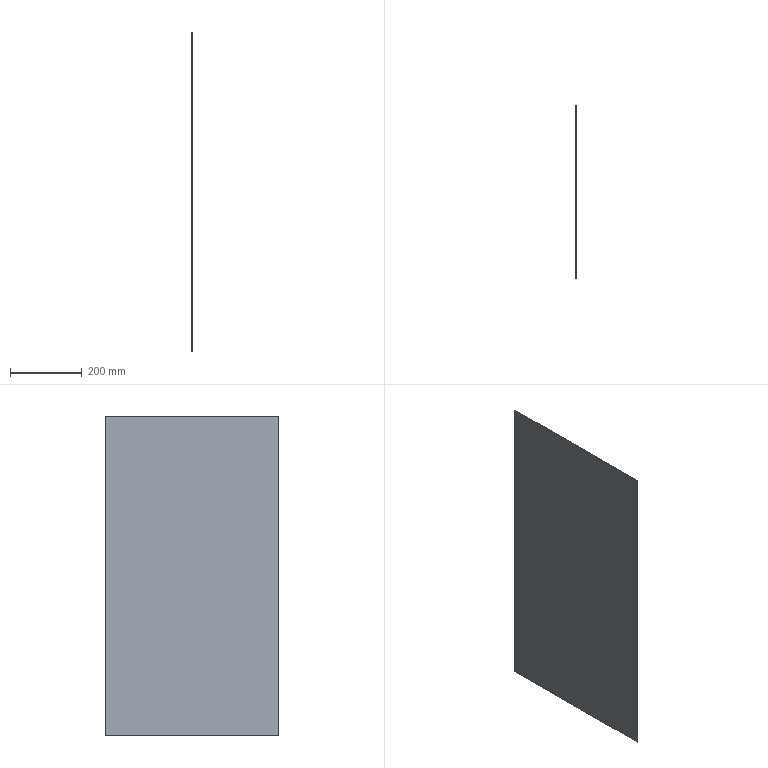Part | STEP file | Guide wheel mechanism revised.sldasm-Part-29 | 1 solid | 6 faces | box 1.2 x 481.99 x 890 mm | volume 514765 mm3 | plane 6
STEP:
#1=CARTESIAN_POINT('',(-485.,1910.,-445.));
#2=VERTEX_POINT('',#1);
#3=CARTESIAN_POINT('',(-485.,1428.01,-445.));
#4=VERTEX_POINT('',#3);
#5=CARTESIAN_POINT('',(-485.,1910.,-445.));
#6=DIRECTION('',(0.,-1.,0.));
#7=VECTOR('',#6,1000.);
#8=LINE('',#5,#7);
#9=EDGE_CURVE('',#2,#4,#8,.T.);
#10=ORIENTED_EDGE('',*,*,#9,.F.);
#11=CARTESIAN_POINT('',(-483.8,1910.,-445.));
#12=VERTEX_POINT('',#11);
#13=CARTESIAN_POINT('',(-483.8,1910.,-445.));
#14=DIRECTION('',(-1.,0.,0.));
#15=VECTOR('',#14,1000.);
#16=LINE('',#13,#15);
#17=EDGE_CURVE('',#12,#2,#16,.T.);
#18=ORIENTED_EDGE('',*,*,#17,.F.);
#19=CARTESIAN_POINT('',(-483.8,1428.01,-445.));
#20=VERTEX_POINT('',#19);
#21=CARTESIAN_POINT('',(-483.8,1910.,-445.));
#22=DIRECTION('',(0.,-1.,0.));
#23=VECTOR('',#22,1000.);
#24=LINE('',#21,#23);
#25=EDGE_CURVE('',#12,#20,#24,.T.);
#26=ORIENTED_EDGE('',*,*,#25,.T.);
#27=CARTESIAN_POINT('',(-483.8,1428.01,-445.));
#28=DIRECTION('',(-1.,0.,0.));
#29=VECTOR('',#28,1000.);
#30=LINE('',#27,#29);
#31=EDGE_CURVE('',#20,#4,#30,.T.);
#32=ORIENTED_EDGE('',*,*,#31,.T.);
#33=EDGE_LOOP('',(#10,#18,#26,#32));
#34=FACE_OUTER_BOUND('',#33,.T.);
#35=CARTESIAN_POINT('',(-483.8,1910.,-445.));
#36=DIRECTION('',(0.,0.,-1.));
#37=DIRECTION('',(0.,1.,0.));
#38=AXIS2_PLACEMENT_3D('',#35,#36,#37);
#39=PLANE('',#38);
#40=ADVANCED_FACE('',(#34),#39,.T.);
#41=CARTESIAN_POINT('',(-485.,1910.,445.));
#42=VERTEX_POINT('',#41);
#43=CARTESIAN_POINT('',(-485.,1910.,-445.));
#44=DIRECTION('',(0.,0.,-1.));
#45=VECTOR('',#44,1000.);
#46=LINE('',#43,#45);
#47=EDGE_CURVE('',#42,#2,#46,.T.);
#48=ORIENTED_EDGE('',*,*,#47,.F.);
#49=CARTESIAN_POINT('',(-483.8,1910.,445.));
#50=VERTEX_POINT('',#49);
#51=CARTESIAN_POINT('',(-483.8,1910.,445.));
#52=DIRECTION('',(-1.,0.,0.));
#53=VECTOR('',#52,1000.);
#54=LINE('',#51,#53);
#55=EDGE_CURVE('',#50,#42,#54,.T.);
#56=ORIENTED_EDGE('',*,*,#55,.F.);
#57=CARTESIAN_POINT('',(-483.8,1910.,-445.));
#58=DIRECTION('',(0.,0.,-1.));
#59=VECTOR('',#58,1000.);
#60=LINE('',#57,#59);
#61=EDGE_CURVE('',#50,#12,#60,.T.);
#62=ORIENTED_EDGE('',*,*,#61,.T.);
#63=ORIENTED_EDGE('',*,*,#17,.T.);
#64=EDGE_LOOP('',(#48,#56,#62,#63));
#65=FACE_OUTER_BOUND('',#64,.T.);
#66=CARTESIAN_POINT('',(-483.8,1910.,-445.));
#67=DIRECTION('',(0.,1.,0.));
#68=DIRECTION('',(0.,0.,1.));
#69=AXIS2_PLACEMENT_3D('',#66,#67,#68);
#70=PLANE('',#69);
#71=ADVANCED_FACE('',(#65),#70,.T.);
#72=CARTESIAN_POINT('',(-485.,1428.01,445.));
#73=VERTEX_POINT('',#72);
#74=CARTESIAN_POINT('',(-485.,1910.,445.));
#75=DIRECTION('',(0.,1.,0.));
#76=VECTOR('',#75,1000.);
#77=LINE('',#74,#76);
#78=EDGE_CURVE('',#73,#42,#77,.T.);
#79=ORIENTED_EDGE('',*,*,#78,.F.);
#80=CARTESIAN_POINT('',(-483.8,1428.01,445.));
#81=VERTEX_POINT('',#80);
#82=CARTESIAN_POINT('',(-483.8,1428.01,445.));
#83=DIRECTION('',(-1.,0.,0.));
#84=VECTOR('',#83,1000.);
#85=LINE('',#82,#84);
#86=EDGE_CURVE('',#81,#73,#85,.T.);
#87=ORIENTED_EDGE('',*,*,#86,.F.);
#88=CARTESIAN_POINT('',(-483.8,1910.,445.));
#89=DIRECTION('',(0.,1.,0.));
#90=VECTOR('',#89,1000.);
#91=LINE('',#88,#90);
#92=EDGE_CURVE('',#81,#50,#91,.T.);
#93=ORIENTED_EDGE('',*,*,#92,.T.);
#94=ORIENTED_EDGE('',*,*,#55,.T.);
#95=EDGE_LOOP('',(#79,#87,#93,#94));
#96=FACE_OUTER_BOUND('',#95,.T.);
#97=CARTESIAN_POINT('',(-483.8,1910.,445.));
#98=DIRECTION('',(0.,0.,1.));
#99=DIRECTION('',(1.,0.,0.));
#100=AXIS2_PLACEMENT_3D('',#97,#98,#99);
#101=PLANE('',#100);
#102=ADVANCED_FACE('',(#96),#101,.T.);
#103=CARTESIAN_POINT('',(-485.,1428.01,-445.));
#104=DIRECTION('',(0.,0.,1.));
#105=VECTOR('',#104,1000.);
#106=LINE('',#103,#105);
#107=EDGE_CURVE('',#4,#73,#106,.T.);
#108=ORIENTED_EDGE('',*,*,#107,.F.);
#109=ORIENTED_EDGE('',*,*,#31,.F.);
#110=CARTESIAN_POINT('',(-483.8,1428.01,-445.));
#111=DIRECTION('',(0.,0.,1.));
#112=VECTOR('',#111,1000.);
#113=LINE('',#110,#112);
#114=EDGE_CURVE('',#20,#81,#113,.T.);
#115=ORIENTED_EDGE('',*,*,#114,.T.);
#116=ORIENTED_EDGE('',*,*,#86,.T.);
#117=EDGE_LOOP('',(#108,#109,#115,#116));
#118=FACE_OUTER_BOUND('',#117,.T.);
#119=CARTESIAN_POINT('',(-483.8,1428.01,-445.));
#120=DIRECTION('',(0.,-1.,0.));
#121=DIRECTION('',(0.,0.,-1.));
#122=AXIS2_PLACEMENT_3D('',#119,#120,#121);
#123=PLANE('',#122);
#124=ADVANCED_FACE('',(#118),#123,.T.);
#125=ORIENTED_EDGE('',*,*,#25,.F.);
#126=ORIENTED_EDGE('',*,*,#61,.F.);
#127=ORIENTED_EDGE('',*,*,#92,.F.);
#128=ORIENTED_EDGE('',*,*,#114,.F.);
#129=EDGE_LOOP('',(#125,#126,#127,#128));
#130=FACE_OUTER_BOUND('',#129,.T.);
#131=CARTESIAN_POINT('',(-483.8,0.,0.));
#132=DIRECTION('',(-1.,0.,0.));
#133=DIRECTION('',(0.,0.,1.));
#134=AXIS2_PLACEMENT_3D('',#131,#132,#133);
#135=PLANE('',#134);
#136=ADVANCED_FACE('',(#130),#135,.F.);
#137=ORIENTED_EDGE('',*,*,#9,.T.);
#138=ORIENTED_EDGE('',*,*,#107,.T.);
#139=ORIENTED_EDGE('',*,*,#78,.T.);
#140=ORIENTED_EDGE('',*,*,#47,.T.);
#141=EDGE_LOOP('',(#137,#138,#139,#140));
#142=FACE_OUTER_BOUND('',#141,.T.);
#143=CARTESIAN_POINT('',(-485.,0.,0.));
#144=DIRECTION('',(-1.,0.,0.));
#145=DIRECTION('',(0.,0.,1.));
#146=AXIS2_PLACEMENT_3D('',#143,#144,#145);
#147=PLANE('',#146);
#148=ADVANCED_FACE('',(#142),#147,.T.);
#149=CLOSED_SHELL('',(#40,#71,#102,#124,#136,#148));
#150=MANIFOLD_SOLID_BREP('',#149);
#151=CARTESIAN_POINT('',(0.,0.,0.));
#152=DIRECTION('',(0.,0.,1.));
#153=DIRECTION('',(1.,0.,0.));
#154=AXIS2_PLACEMENT_3D('',#151,#152,#153);
#155=(LENGTH_UNIT()NAMED_UNIT(*)SI_UNIT(.MILLI.,.METRE.));
#156=UNCERTAINTY_MEASURE_WITH_UNIT(LENGTH_MEASURE(0.00001),#155,'','');
#157=(NAMED_UNIT(*)PLANE_ANGLE_UNIT()SI_UNIT($,.RADIAN.));
#158=(NAMED_UNIT(*)SI_UNIT($,.STERADIAN.)SOLID_ANGLE_UNIT());
#159=(GEOMETRIC_REPRESENTATION_CONTEXT(3)GLOBAL_UNCERTAINTY_ASSIGNED_CONTEXT((#156))GLOBAL_UNIT_ASSIGNED_CONTEXT((#155,#157,#158))REPRESENTATION_CONTEXT('',''));
#160=ADVANCED_BREP_SHAPE_REPRESENTATION('',(#150,#154),#159);